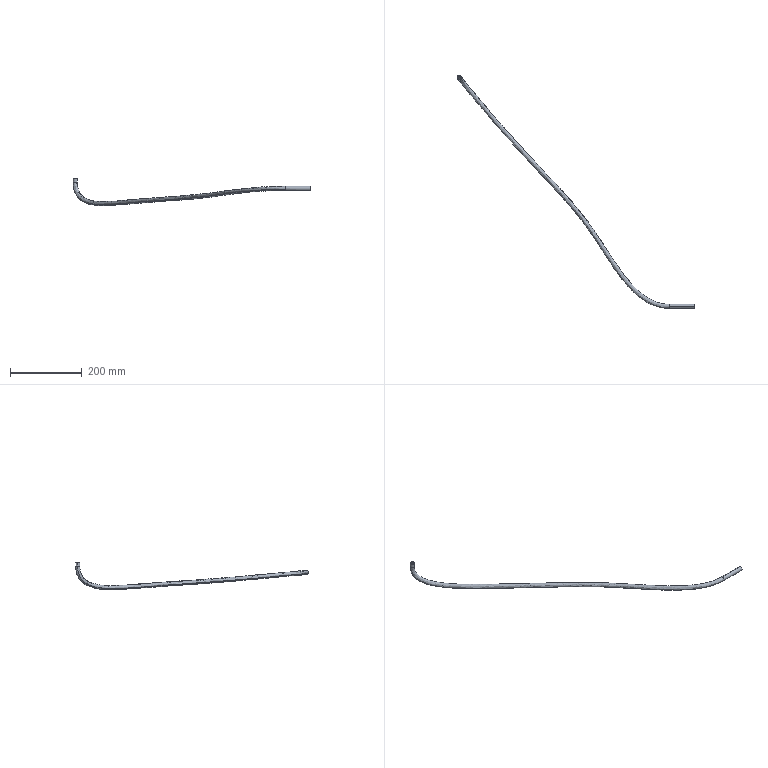Part | SolidWorks | features 3DProfileFeature 2, Sweep 1 | 1 solid | 14 faces | box 662.345 x 648.516 x 77.026 mm | volume 34265 mm3 | cylinder 8 | spline 4 | plane 2 | commonest cylinder face diameters 10 x4 12 x4